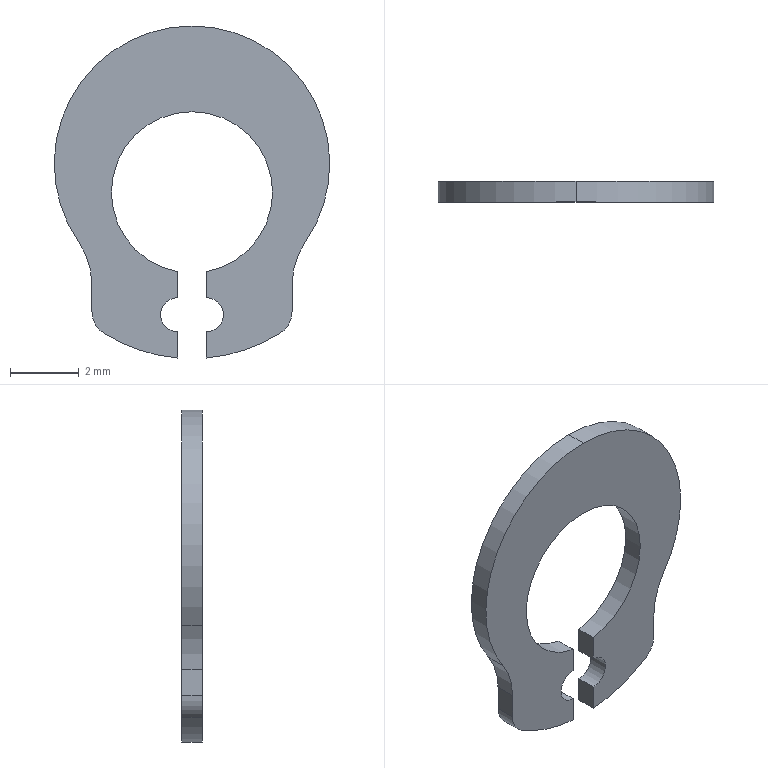Part | SolidWorks | features BaseBody 1 | 1 solid | 20 faces | box 8.033 x 0.6 x 9.682 mm | volume 24.423 mm3 | cylinder 12 | plane 8 | commonest cylinder face diameters 1 x2 1.5 x2 4.5 x2 4.7 x2 8.033 x2 9.7 x2
STEP:
#1=CARTESIAN_POINT('',(0.4167,-0.6,-2.313));
#2=VERTEX_POINT('',#1);
#3=CARTESIAN_POINT('',(0.,-0.6,2.35));
#4=VERTEX_POINT('',#3);
#5=CARTESIAN_POINT('',(0.,-0.6,0.));
#6=DIRECTION('',(0.,-1.,0.));
#7=DIRECTION('',(0.,0.,-1.));
#8=AXIS2_PLACEMENT_3D('',#5,#6,#7);
#9=CIRCLE('',#8,2.35);
#10=EDGE_CURVE('',#2,#4,#9,.T.);
#11=ORIENTED_EDGE('',*,*,#10,.T.);
#12=CARTESIAN_POINT('',(0.,0.,2.35));
#13=VERTEX_POINT('',#12);
#14=CARTESIAN_POINT('',(0.,-0.6,2.35));
#15=DIRECTION('',(0.,1.,0.));
#16=VECTOR('',#15,1000.);
#17=LINE('',#14,#16);
#18=EDGE_CURVE('',#4,#13,#17,.T.);
#19=ORIENTED_EDGE('',*,*,#18,.T.);
#20=CARTESIAN_POINT('',(0.4167,0.,-2.313));
#21=VERTEX_POINT('',#20);
#22=CARTESIAN_POINT('',(0.,0.,0.));
#23=DIRECTION('',(0.,-1.,0.));
#24=DIRECTION('',(0.,0.,-1.));
#25=AXIS2_PLACEMENT_3D('',#22,#23,#24);
#26=CIRCLE('',#25,2.35);
#27=EDGE_CURVE('',#21,#13,#26,.T.);
#28=ORIENTED_EDGE('',*,*,#27,.F.);
#29=CARTESIAN_POINT('',(0.4167,-0.6,-2.313));
#30=DIRECTION('',(0.,1.,0.));
#31=VECTOR('',#30,1000.);
#32=LINE('',#29,#31);
#33=EDGE_CURVE('',#2,#21,#32,.T.);
#34=ORIENTED_EDGE('',*,*,#33,.F.);
#35=EDGE_LOOP('',(#11,#19,#28,#34));
#36=FACE_OUTER_BOUND('',#35,.T.);
#37=CARTESIAN_POINT('',(0.,-0.6,0.));
#38=DIRECTION('',(0.,1.,0.));
#39=DIRECTION('',(0.,0.,1.));
#40=AXIS2_PLACEMENT_3D('',#37,#38,#39);
#41=CYLINDRICAL_SURFACE('',#40,2.35);
#42=ADVANCED_FACE('',(#36),#41,.F.);
#43=CARTESIAN_POINT('',(-3.312,-0.6,-1.44));
#44=VERTEX_POINT('',#43);
#45=CARTESIAN_POINT('',(0.,-0.6,4.85));
#46=VERTEX_POINT('',#45);
#47=CARTESIAN_POINT('',(0.,-0.6,0.8333));
#48=DIRECTION('',(0.,1.,0.));
#49=DIRECTION('',(0.,0.,-1.));
#50=AXIS2_PLACEMENT_3D('',#47,#48,#49);
#51=CIRCLE('',#50,4.017);
#52=EDGE_CURVE('',#44,#46,#51,.T.);
#53=ORIENTED_EDGE('',*,*,#52,.T.);
#54=CARTESIAN_POINT('',(0.,0.,4.85));
#55=VERTEX_POINT('',#54);
#56=CARTESIAN_POINT('',(0.,-0.6,4.85));
#57=DIRECTION('',(0.,1.,0.));
#58=VECTOR('',#57,1000.);
#59=LINE('',#56,#58);
#60=EDGE_CURVE('',#46,#55,#59,.T.);
#61=ORIENTED_EDGE('',*,*,#60,.T.);
#62=CARTESIAN_POINT('',(-3.312,0.,-1.44));
#63=VERTEX_POINT('',#62);
#64=CARTESIAN_POINT('',(0.,0.,0.8333));
#65=DIRECTION('',(0.,1.,0.));
#66=DIRECTION('',(0.,0.,-1.));
#67=AXIS2_PLACEMENT_3D('',#64,#65,#66);
#68=CIRCLE('',#67,4.017);
#69=EDGE_CURVE('',#63,#55,#68,.T.);
#70=ORIENTED_EDGE('',*,*,#69,.F.);
#71=CARTESIAN_POINT('',(-3.312,-0.6,-1.44));
#72=DIRECTION('',(0.,-1.,0.));
#73=VECTOR('',#72,1000.);
#74=LINE('',#71,#73);
#75=EDGE_CURVE('',#63,#44,#74,.T.);
#76=ORIENTED_EDGE('',*,*,#75,.T.);
#77=EDGE_LOOP('',(#53,#61,#70,#76));
#78=FACE_OUTER_BOUND('',#77,.T.);
#79=CARTESIAN_POINT('',(0.,-0.6,0.8333));
#80=DIRECTION('',(0.,1.,0.));
#81=DIRECTION('',(0.,0.,1.));
#82=AXIS2_PLACEMENT_3D('',#79,#80,#81);
#83=CYLINDRICAL_SURFACE('',#82,4.017);
#84=ADVANCED_FACE('',(#78),#83,.T.);
#85=CARTESIAN_POINT('',(-2.917,-0.6,-3.481));
#86=VERTEX_POINT('',#85);
#87=CARTESIAN_POINT('',(-2.563,-0.6,-4.117));
#88=VERTEX_POINT('',#87);
#89=CARTESIAN_POINT('',(-2.167,-0.6,-3.481));
#90=DIRECTION('',(0.,-1.,0.));
#91=DIRECTION('',(0.,0.,-1.));
#92=AXIS2_PLACEMENT_3D('',#89,#90,#91);
#93=CIRCLE('',#92,0.75);
#94=EDGE_CURVE('',#86,#88,#93,.T.);
#95=ORIENTED_EDGE('',*,*,#94,.F.);
#96=CARTESIAN_POINT('',(-2.917,0.,-3.481));
#97=VERTEX_POINT('',#96);
#98=CARTESIAN_POINT('',(-2.917,-0.6,-3.481));
#99=DIRECTION('',(0.,-1.,0.));
#100=VECTOR('',#99,1000.);
#101=LINE('',#98,#100);
#102=EDGE_CURVE('',#97,#86,#101,.T.);
#103=ORIENTED_EDGE('',*,*,#102,.F.);
#104=CARTESIAN_POINT('',(-2.563,0.,-4.117));
#105=VERTEX_POINT('',#104);
#106=CARTESIAN_POINT('',(-2.167,0.,-3.481));
#107=DIRECTION('',(0.,1.,0.));
#108=DIRECTION('',(0.,0.,-1.));
#109=AXIS2_PLACEMENT_3D('',#106,#107,#108);
#110=CIRCLE('',#109,0.75);
#111=EDGE_CURVE('',#105,#97,#110,.T.);
#112=ORIENTED_EDGE('',*,*,#111,.F.);
#113=CARTESIAN_POINT('',(-2.563,-0.6,-4.117));
#114=DIRECTION('',(0.,1.,0.));
#115=VECTOR('',#114,1000.);
#116=LINE('',#113,#115);
#117=EDGE_CURVE('',#88,#105,#116,.T.);
#118=ORIENTED_EDGE('',*,*,#117,.F.);
#119=EDGE_LOOP('',(#95,#103,#112,#118));
#120=FACE_OUTER_BOUND('',#119,.T.);
#121=CARTESIAN_POINT('',(-2.167,-0.6,-3.481));
#122=DIRECTION('',(0.,1.,0.));
#123=DIRECTION('',(0.,0.,1.));
#124=AXIS2_PLACEMENT_3D('',#121,#122,#123);
#125=CYLINDRICAL_SURFACE('',#124,0.75);
#126=ADVANCED_FACE('',(#120),#125,.T.);
#127=CARTESIAN_POINT('',(2.563,-0.6,-4.117));
#128=VERTEX_POINT('',#127);
#129=CARTESIAN_POINT('',(2.917,-0.6,-3.481));
#130=VERTEX_POINT('',#129);
#131=CARTESIAN_POINT('',(2.167,-0.6,-3.481));
#132=DIRECTION('',(0.,-1.,0.));
#133=DIRECTION('',(0.,0.,-1.));
#134=AXIS2_PLACEMENT_3D('',#131,#132,#133);
#135=CIRCLE('',#134,0.75);
#136=EDGE_CURVE('',#128,#130,#135,.T.);
#137=ORIENTED_EDGE('',*,*,#136,.F.);
#138=CARTESIAN_POINT('',(2.563,0.,-4.117));
#139=VERTEX_POINT('',#138);
#140=CARTESIAN_POINT('',(2.563,-0.6,-4.117));
#141=DIRECTION('',(0.,-1.,0.));
#142=VECTOR('',#141,1000.);
#143=LINE('',#140,#142);
#144=EDGE_CURVE('',#139,#128,#143,.T.);
#145=ORIENTED_EDGE('',*,*,#144,.F.);
#146=CARTESIAN_POINT('',(2.917,0.,-3.481));
#147=VERTEX_POINT('',#146);
#148=CARTESIAN_POINT('',(2.167,0.,-3.481));
#149=DIRECTION('',(0.,1.,0.));
#150=DIRECTION('',(0.,0.,-1.));
#151=AXIS2_PLACEMENT_3D('',#148,#149,#150);
#152=CIRCLE('',#151,0.75);
#153=EDGE_CURVE('',#147,#139,#152,.T.);
#154=ORIENTED_EDGE('',*,*,#153,.F.);
#155=CARTESIAN_POINT('',(2.917,-0.6,-3.481));
#156=DIRECTION('',(0.,1.,0.));
#157=VECTOR('',#156,1000.);
#158=LINE('',#155,#157);
#159=EDGE_CURVE('',#130,#147,#158,.T.);
#160=ORIENTED_EDGE('',*,*,#159,.F.);
#161=EDGE_LOOP('',(#137,#145,#154,#160));
#162=FACE_OUTER_BOUND('',#161,.T.);
#163=CARTESIAN_POINT('',(2.167,-0.6,-3.481));
#164=DIRECTION('',(0.,1.,0.));
#165=DIRECTION('',(0.,0.,1.));
#166=AXIS2_PLACEMENT_3D('',#163,#164,#165);
#167=CYLINDRICAL_SURFACE('',#166,0.75);
#168=ADVANCED_FACE('',(#162),#167,.T.);
#169=CARTESIAN_POINT('',(-2.917,-0.6,-2.713));
#170=VERTEX_POINT('',#169);
#171=CARTESIAN_POINT('',(-5.167,-0.6,-2.713));
#172=DIRECTION('',(0.,1.,0.));
#173=DIRECTION('',(0.,0.,-1.));
#174=AXIS2_PLACEMENT_3D('',#171,#172,#173);
#175=CIRCLE('',#174,2.25);
#176=EDGE_CURVE('',#44,#170,#175,.T.);
#177=ORIENTED_EDGE('',*,*,#176,.F.);
#178=ORIENTED_EDGE('',*,*,#75,.F.);
#179=CARTESIAN_POINT('',(-2.917,0.,-2.713));
#180=VERTEX_POINT('',#179);
#181=CARTESIAN_POINT('',(-5.167,0.,-2.713));
#182=DIRECTION('',(0.,-1.,0.));
#183=DIRECTION('',(0.,0.,-1.));
#184=AXIS2_PLACEMENT_3D('',#181,#182,#183);
#185=CIRCLE('',#184,2.25);
#186=EDGE_CURVE('',#180,#63,#185,.T.);
#187=ORIENTED_EDGE('',*,*,#186,.F.);
#188=CARTESIAN_POINT('',(-2.917,0.,-2.713));
#189=DIRECTION('',(0.,1.,0.));
#190=VECTOR('',#189,1000.);
#191=LINE('',#188,#190);
#192=EDGE_CURVE('',#170,#180,#191,.T.);
#193=ORIENTED_EDGE('',*,*,#192,.F.);
#194=EDGE_LOOP('',(#177,#178,#187,#193));
#195=FACE_OUTER_BOUND('',#194,.T.);
#196=CARTESIAN_POINT('',(-5.167,-0.6,-2.713));
#197=DIRECTION('',(0.,1.,0.));
#198=DIRECTION('',(0.,0.,1.));
#199=AXIS2_PLACEMENT_3D('',#196,#197,#198);
#200=CYLINDRICAL_SURFACE('',#199,2.25);
#201=ADVANCED_FACE('',(#195),#200,.F.);
#202=CARTESIAN_POINT('',(2.917,-0.6,-2.713));
#203=VERTEX_POINT('',#202);
#204=CARTESIAN_POINT('',(3.312,-0.6,-1.44));
#205=VERTEX_POINT('',#204);
#206=CARTESIAN_POINT('',(5.167,-0.6,-2.713));
#207=DIRECTION('',(0.,1.,0.));
#208=DIRECTION('',(0.,0.,-1.));
#209=AXIS2_PLACEMENT_3D('',#206,#207,#208);
#210=CIRCLE('',#209,2.25);
#211=EDGE_CURVE('',#203,#205,#210,.T.);
#212=ORIENTED_EDGE('',*,*,#211,.F.);
#213=CARTESIAN_POINT('',(2.917,0.,-2.713));
#214=VERTEX_POINT('',#213);
#215=CARTESIAN_POINT('',(2.917,-0.6,-2.713));
#216=DIRECTION('',(0.,-1.,0.));
#217=VECTOR('',#216,1000.);
#218=LINE('',#215,#217);
#219=EDGE_CURVE('',#214,#203,#218,.T.);
#220=ORIENTED_EDGE('',*,*,#219,.F.);
#221=CARTESIAN_POINT('',(3.312,0.,-1.44));
#222=VERTEX_POINT('',#221);
#223=CARTESIAN_POINT('',(5.167,0.,-2.713));
#224=DIRECTION('',(0.,-1.,0.));
#225=DIRECTION('',(0.,0.,-1.));
#226=AXIS2_PLACEMENT_3D('',#223,#224,#225);
#227=CIRCLE('',#226,2.25);
#228=EDGE_CURVE('',#222,#214,#227,.T.);
#229=ORIENTED_EDGE('',*,*,#228,.F.);
#230=CARTESIAN_POINT('',(3.312,-0.6,-1.44));
#231=DIRECTION('',(0.,1.,0.));
#232=VECTOR('',#231,1000.);
#233=LINE('',#230,#232);
#234=EDGE_CURVE('',#205,#222,#233,.T.);
#235=ORIENTED_EDGE('',*,*,#234,.F.);
#236=EDGE_LOOP('',(#212,#220,#229,#235));
#237=FACE_OUTER_BOUND('',#236,.T.);
#238=CARTESIAN_POINT('',(5.167,-0.6,-2.713));
#239=DIRECTION('',(0.,1.,0.));
#240=DIRECTION('',(0.,0.,1.));
#241=AXIS2_PLACEMENT_3D('',#238,#239,#240);
#242=CYLINDRICAL_SURFACE('',#241,2.25);
#243=ADVANCED_FACE('',(#237),#242,.F.);
#244=CARTESIAN_POINT('',(-0.4167,-0.6,-4.072));
#245=VERTEX_POINT('',#244);
#246=CARTESIAN_POINT('',(-0.4167,-0.6,-3.072));
#247=VERTEX_POINT('',#246);
#248=CARTESIAN_POINT('',(-0.4167,-0.6,-3.572));
#249=DIRECTION('',(0.,1.,0.));
#250=DIRECTION('',(0.,0.,-1.));
#251=AXIS2_PLACEMENT_3D('',#248,#249,#250);
#252=CIRCLE('',#251,0.5);
#253=EDGE_CURVE('',#245,#247,#252,.T.);
#254=ORIENTED_EDGE('',*,*,#253,.F.);
#255=CARTESIAN_POINT('',(-0.4167,0.,-4.072));
#256=VERTEX_POINT('',#255);
#257=CARTESIAN_POINT('',(-0.4167,11.995,-4.072));
#258=DIRECTION('',(0.,-1.,0.));
#259=VECTOR('',#258,1000.);
#260=LINE('',#257,#259);
#261=EDGE_CURVE('',#256,#245,#260,.T.);
#262=ORIENTED_EDGE('',*,*,#261,.F.);
#263=CARTESIAN_POINT('',(-0.4167,0.,-3.072));
#264=VERTEX_POINT('',#263);
#265=CARTESIAN_POINT('',(-0.4167,0.,-3.572));
#266=DIRECTION('',(0.,1.,0.));
#267=DIRECTION('',(0.,0.,-1.));
#268=AXIS2_PLACEMENT_3D('',#265,#266,#267);
#269=CIRCLE('',#268,0.5);
#270=EDGE_CURVE('',#256,#264,#269,.T.);
#271=ORIENTED_EDGE('',*,*,#270,.T.);
#272=CARTESIAN_POINT('',(-0.4167,11.995,-3.072));
#273=DIRECTION('',(0.,1.,0.));
#274=VECTOR('',#273,1000.);
#275=LINE('',#272,#274);
#276=EDGE_CURVE('',#247,#264,#275,.T.);
#277=ORIENTED_EDGE('',*,*,#276,.F.);
#278=EDGE_LOOP('',(#254,#262,#271,#277));
#279=FACE_OUTER_BOUND('',#278,.T.);
#280=CARTESIAN_POINT('',(-0.4167,11.995,-3.572));
#281=DIRECTION('',(0.,-1.,0.));
#282=DIRECTION('',(0.,0.,-1.));
#283=AXIS2_PLACEMENT_3D('',#280,#281,#282);
#284=CYLINDRICAL_SURFACE('',#283,0.5);
#285=ADVANCED_FACE('',(#279),#284,.F.);
#286=CARTESIAN_POINT('',(0.4167,-0.6,-3.072));
#287=VERTEX_POINT('',#286);
#288=CARTESIAN_POINT('',(0.4167,-0.6,-4.072));
#289=VERTEX_POINT('',#288);
#290=CARTESIAN_POINT('',(0.4167,-0.6,-3.572));
#291=DIRECTION('',(0.,1.,0.));
#292=DIRECTION('',(0.,0.,-1.));
#293=AXIS2_PLACEMENT_3D('',#290,#291,#292);
#294=CIRCLE('',#293,0.5);
#295=EDGE_CURVE('',#287,#289,#294,.T.);
#296=ORIENTED_EDGE('',*,*,#295,.F.);
#297=CARTESIAN_POINT('',(0.4167,0.,-3.072));
#298=VERTEX_POINT('',#297);
#299=CARTESIAN_POINT('',(0.4167,11.995,-3.072));
#300=DIRECTION('',(0.,-1.,0.));
#301=VECTOR('',#300,1000.);
#302=LINE('',#299,#301);
#303=EDGE_CURVE('',#298,#287,#302,.T.);
#304=ORIENTED_EDGE('',*,*,#303,.F.);
#305=CARTESIAN_POINT('',(0.4167,0.,-4.072));
#306=VERTEX_POINT('',#305);
#307=CARTESIAN_POINT('',(0.4167,0.,-3.572));
#308=DIRECTION('',(0.,1.,0.));
#309=DIRECTION('',(0.,0.,-1.));
#310=AXIS2_PLACEMENT_3D('',#307,#308,#309);
#311=CIRCLE('',#310,0.5);
#312=EDGE_CURVE('',#298,#306,#311,.T.);
#313=ORIENTED_EDGE('',*,*,#312,.T.);
#314=CARTESIAN_POINT('',(0.4167,11.995,-4.072));
#315=DIRECTION('',(0.,1.,0.));
#316=VECTOR('',#315,1000.);
#317=LINE('',#314,#316);
#318=EDGE_CURVE('',#289,#306,#317,.T.);
#319=ORIENTED_EDGE('',*,*,#318,.F.);
#320=EDGE_LOOP('',(#296,#304,#313,#319));
#321=FACE_OUTER_BOUND('',#320,.T.);
#322=CARTESIAN_POINT('',(0.4167,11.995,-3.572));
#323=DIRECTION('',(0.,-1.,0.));
#324=DIRECTION('',(0.,0.,-1.));
#325=AXIS2_PLACEMENT_3D('',#322,#323,#324);
#326=CYLINDRICAL_SURFACE('',#325,0.5);
#327=ADVANCED_FACE('',(#321),#326,.F.);
#328=CARTESIAN_POINT('',(-0.4167,0.,-4.832));
#329=VERTEX_POINT('',#328);
#330=CARTESIAN_POINT('',(0.,0.,0.));
#331=DIRECTION('',(0.,1.,0.));
#332=DIRECTION('',(1.,0.,0.));
#333=AXIS2_PLACEMENT_3D('',#330,#331,#332);
#334=CIRCLE('',#333,4.85);
#335=EDGE_CURVE('',#329,#105,#334,.T.);
#336=ORIENTED_EDGE('',*,*,#335,.T.);
#337=ORIENTED_EDGE('',*,*,#111,.T.);
#338=CARTESIAN_POINT('',(-2.917,0.,-1.928));
#339=DIRECTION('',(0.,0.,1.));
#340=VECTOR('',#339,1000.);
#341=LINE('',#338,#340);
#342=EDGE_CURVE('',#97,#180,#341,.T.);
#343=ORIENTED_EDGE('',*,*,#342,.T.);
#344=ORIENTED_EDGE('',*,*,#186,.T.);
#345=ORIENTED_EDGE('',*,*,#69,.T.);
#346=CARTESIAN_POINT('',(0.,0.,0.8333));
#347=DIRECTION('',(0.,1.,0.));
#348=DIRECTION('',(0.,0.,-1.));
#349=AXIS2_PLACEMENT_3D('',#346,#347,#348);
#350=CIRCLE('',#349,4.017);
#351=EDGE_CURVE('',#55,#222,#350,.T.);
#352=ORIENTED_EDGE('',*,*,#351,.T.);
#353=ORIENTED_EDGE('',*,*,#228,.T.);
#354=CARTESIAN_POINT('',(2.917,0.,-1.928));
#355=DIRECTION('',(0.,0.,-1.));
#356=VECTOR('',#355,1000.);
#357=LINE('',#354,#356);
#358=EDGE_CURVE('',#214,#147,#357,.T.);
#359=ORIENTED_EDGE('',*,*,#358,.T.);
#360=ORIENTED_EDGE('',*,*,#153,.T.);
#361=CARTESIAN_POINT('',(0.4167,0.,-4.832));
#362=VERTEX_POINT('',#361);
#363=CARTESIAN_POINT('',(0.,0.,0.));
#364=DIRECTION('',(0.,1.,0.));
#365=DIRECTION('',(1.,0.,0.));
#366=AXIS2_PLACEMENT_3D('',#363,#364,#365);
#367=CIRCLE('',#366,4.85);
#368=EDGE_CURVE('',#139,#362,#367,.T.);
#369=ORIENTED_EDGE('',*,*,#368,.T.);
#370=CARTESIAN_POINT('',(0.4167,0.,-2.313));
#371=DIRECTION('',(0.,0.,1.));
#372=VECTOR('',#371,1000.);
#373=LINE('',#370,#372);
#374=EDGE_CURVE('',#362,#306,#373,.T.);
#375=ORIENTED_EDGE('',*,*,#374,.T.);
#376=ORIENTED_EDGE('',*,*,#312,.F.);
#377=CARTESIAN_POINT('',(0.4167,0.,-2.313));
#378=DIRECTION('',(0.,0.,1.));
#379=VECTOR('',#378,1000.);
#380=LINE('',#377,#379);
#381=EDGE_CURVE('',#298,#21,#380,.T.);
#382=ORIENTED_EDGE('',*,*,#381,.T.);
#383=ORIENTED_EDGE('',*,*,#27,.T.);
#384=CARTESIAN_POINT('',(-0.4167,0.,-2.313));
#385=VERTEX_POINT('',#384);
#386=CARTESIAN_POINT('',(0.,0.,0.));
#387=DIRECTION('',(0.,-1.,0.));
#388=DIRECTION('',(0.,0.,-1.));
#389=AXIS2_PLACEMENT_3D('',#386,#387,#388);
#390=CIRCLE('',#389,2.35);
#391=EDGE_CURVE('',#13,#385,#390,.T.);
#392=ORIENTED_EDGE('',*,*,#391,.T.);
#393=CARTESIAN_POINT('',(-0.4167,0.,-2.313));
#394=DIRECTION('',(0.,0.,-1.));
#395=VECTOR('',#394,1000.);
#396=LINE('',#393,#395);
#397=EDGE_CURVE('',#385,#264,#396,.T.);
#398=ORIENTED_EDGE('',*,*,#397,.T.);
#399=ORIENTED_EDGE('',*,*,#270,.F.);
#400=CARTESIAN_POINT('',(-0.4167,0.,-2.313));
#401=DIRECTION('',(0.,0.,-1.));
#402=VECTOR('',#401,1000.);
#403=LINE('',#400,#402);
#404=EDGE_CURVE('',#256,#329,#403,.T.);
#405=ORIENTED_EDGE('',*,*,#404,.T.);
#406=EDGE_LOOP('',(#336,#337,#343,#344,#345,#352,#353,#359,#360,#369,#375,#376,#382,#383,#392,#398,#399,#405));
#407=FACE_OUTER_BOUND('',#406,.T.);
#408=CARTESIAN_POINT('',(0.,0.,0.));
#409=DIRECTION('',(0.,-1.,0.));
#410=DIRECTION('',(0.,0.,-1.));
#411=AXIS2_PLACEMENT_3D('',#408,#409,#410);
#412=PLANE('',#411);
#413=ADVANCED_FACE('',(#407),#412,.F.);
#414=CARTESIAN_POINT('',(-2.917,-0.6,-1.928));
#415=DIRECTION('',(0.,0.,1.));
#416=VECTOR('',#415,1000.);
#417=LINE('',#414,#416);
#418=EDGE_CURVE('',#86,#170,#417,.T.);
#419=ORIENTED_EDGE('',*,*,#418,.F.);
#420=ORIENTED_EDGE('',*,*,#94,.T.);
#421=CARTESIAN_POINT('',(-0.4167,-0.6,-4.832));
#422=VERTEX_POINT('',#421);
#423=CARTESIAN_POINT('',(0.,-0.6,0.));
#424=DIRECTION('',(0.,1.,0.));
#425=DIRECTION('',(1.,0.,0.));
#426=AXIS2_PLACEMENT_3D('',#423,#424,#425);
#427=CIRCLE('',#426,4.85);
#428=EDGE_CURVE('',#422,#88,#427,.T.);
#429=ORIENTED_EDGE('',*,*,#428,.F.);
#430=CARTESIAN_POINT('',(-0.4167,-0.6,-2.313));
#431=DIRECTION('',(0.,0.,-1.));
#432=VECTOR('',#431,1000.);
#433=LINE('',#430,#432);
#434=EDGE_CURVE('',#245,#422,#433,.T.);
#435=ORIENTED_EDGE('',*,*,#434,.F.);
#436=ORIENTED_EDGE('',*,*,#253,.T.);
#437=CARTESIAN_POINT('',(-0.4167,-0.6,-2.313));
#438=VERTEX_POINT('',#437);
#439=CARTESIAN_POINT('',(-0.4167,-0.6,-2.313));
#440=DIRECTION('',(0.,0.,-1.));
#441=VECTOR('',#440,1000.);
#442=LINE('',#439,#441);
#443=EDGE_CURVE('',#438,#247,#442,.T.);
#444=ORIENTED_EDGE('',*,*,#443,.F.);
#445=CARTESIAN_POINT('',(0.,-0.6,0.));
#446=DIRECTION('',(0.,-1.,0.));
#447=DIRECTION('',(0.,0.,-1.));
#448=AXIS2_PLACEMENT_3D('',#445,#446,#447);
#449=CIRCLE('',#448,2.35);
#450=EDGE_CURVE('',#4,#438,#449,.T.);
#451=ORIENTED_EDGE('',*,*,#450,.F.);
#452=ORIENTED_EDGE('',*,*,#10,.F.);
#453=CARTESIAN_POINT('',(0.4167,-0.6,-2.313));
#454=DIRECTION('',(0.,0.,1.));
#455=VECTOR('',#454,1000.);
#456=LINE('',#453,#455);
#457=EDGE_CURVE('',#287,#2,#456,.T.);
#458=ORIENTED_EDGE('',*,*,#457,.F.);
#459=ORIENTED_EDGE('',*,*,#295,.T.);
#460=CARTESIAN_POINT('',(0.4167,-0.6,-4.832));
#461=VERTEX_POINT('',#460);
#462=CARTESIAN_POINT('',(0.4167,-0.6,-2.313));
#463=DIRECTION('',(0.,0.,1.));
#464=VECTOR('',#463,1000.);
#465=LINE('',#462,#464);
#466=EDGE_CURVE('',#461,#289,#465,.T.);
#467=ORIENTED_EDGE('',*,*,#466,.F.);
#468=CARTESIAN_POINT('',(0.,-0.6,0.));
#469=DIRECTION('',(0.,1.,0.));
#470=DIRECTION('',(1.,0.,0.));
#471=AXIS2_PLACEMENT_3D('',#468,#469,#470);
#472=CIRCLE('',#471,4.85);
#473=EDGE_CURVE('',#128,#461,#472,.T.);
#474=ORIENTED_EDGE('',*,*,#473,.F.);
#475=ORIENTED_EDGE('',*,*,#136,.T.);
#476=CARTESIAN_POINT('',(2.917,-0.6,-1.928));
#477=DIRECTION('',(0.,0.,-1.));
#478=VECTOR('',#477,1000.);
#479=LINE('',#476,#478);
#480=EDGE_CURVE('',#203,#130,#479,.T.);
#481=ORIENTED_EDGE('',*,*,#480,.F.);
#482=ORIENTED_EDGE('',*,*,#211,.T.);
#483=CARTESIAN_POINT('',(0.,-0.6,0.8333));
#484=DIRECTION('',(0.,1.,0.));
#485=DIRECTION('',(0.,0.,-1.));
#486=AXIS2_PLACEMENT_3D('',#483,#484,#485);
#487=CIRCLE('',#486,4.017);
#488=EDGE_CURVE('',#46,#205,#487,.T.);
#489=ORIENTED_EDGE('',*,*,#488,.F.);
#490=ORIENTED_EDGE('',*,*,#52,.F.);
#491=ORIENTED_EDGE('',*,*,#176,.T.);
#492=EDGE_LOOP('',(#419,#420,#429,#435,#436,#444,#451,#452,#458,#459,#467,#474,#475,#481,#482,#489,#490,#491));
#493=FACE_OUTER_BOUND('',#492,.T.);
#494=CARTESIAN_POINT('',(0.,-0.6,0.));
#495=DIRECTION('',(0.,-1.,0.));
#496=DIRECTION('',(0.,0.,-1.));
#497=AXIS2_PLACEMENT_3D('',#494,#495,#496);
#498=PLANE('',#497);
#499=ADVANCED_FACE('',(#493),#498,.T.);
#500=ORIENTED_EDGE('',*,*,#368,.F.);
#501=ORIENTED_EDGE('',*,*,#144,.T.);
#502=ORIENTED_EDGE('',*,*,#473,.T.);
#503=CARTESIAN_POINT('',(0.4167,-0.6,-4.832));
#504=DIRECTION('',(0.,1.,0.));
#505=VECTOR('',#504,1000.);
#506=LINE('',#503,#505);
#507=EDGE_CURVE('',#461,#362,#506,.T.);
#508=ORIENTED_EDGE('',*,*,#507,.T.);
#509=EDGE_LOOP('',(#500,#501,#502,#508));
#510=FACE_OUTER_BOUND('',#509,.T.);
#511=CARTESIAN_POINT('',(0.,-0.6,0.));
#512=DIRECTION('',(0.,1.,0.));
#513=DIRECTION('',(0.,0.,1.));
#514=AXIS2_PLACEMENT_3D('',#511,#512,#513);
#515=CYLINDRICAL_SURFACE('',#514,4.85);
#516=ADVANCED_FACE('',(#510),#515,.T.);
#517=ORIENTED_EDGE('',*,*,#480,.T.);
#518=ORIENTED_EDGE('',*,*,#159,.T.);
#519=ORIENTED_EDGE('',*,*,#358,.F.);
#520=ORIENTED_EDGE('',*,*,#219,.T.);
#521=EDGE_LOOP('',(#517,#518,#519,#520));
#522=FACE_OUTER_BOUND('',#521,.T.);
#523=CARTESIAN_POINT('',(2.917,-0.6,-1.928));
#524=DIRECTION('',(1.,0.,0.));
#525=DIRECTION('',(0.,0.,-1.));
#526=AXIS2_PLACEMENT_3D('',#523,#524,#525);
#527=PLANE('',#526);
#528=ADVANCED_FACE('',(#522),#527,.T.);
#529=ORIENTED_EDGE('',*,*,#60,.F.);
#530=ORIENTED_EDGE('',*,*,#488,.T.);
#531=ORIENTED_EDGE('',*,*,#234,.T.);
#532=ORIENTED_EDGE('',*,*,#351,.F.);
#533=EDGE_LOOP('',(#529,#530,#531,#532));
#534=FACE_OUTER_BOUND('',#533,.T.);
#535=CARTESIAN_POINT('',(0.,-0.6,0.8333));
#536=DIRECTION('',(0.,1.,0.));
#537=DIRECTION('',(0.,0.,1.));
#538=AXIS2_PLACEMENT_3D('',#535,#536,#537);
#539=CYLINDRICAL_SURFACE('',#538,4.017);
#540=ADVANCED_FACE('',(#534),#539,.T.);
#541=ORIENTED_EDGE('',*,*,#342,.F.);
#542=ORIENTED_EDGE('',*,*,#102,.T.);
#543=ORIENTED_EDGE('',*,*,#418,.T.);
#544=ORIENTED_EDGE('',*,*,#192,.T.);
#545=EDGE_LOOP('',(#541,#542,#543,#544));
#546=FACE_OUTER_BOUND('',#545,.T.);
#547=CARTESIAN_POINT('',(-2.917,-0.6,-1.928));
#548=DIRECTION('',(-1.,0.,0.));
#549=DIRECTION('',(0.,1.,0.));
#550=AXIS2_PLACEMENT_3D('',#547,#548,#549);
#551=PLANE('',#550);
#552=ADVANCED_FACE('',(#546),#551,.T.);
#553=ORIENTED_EDGE('',*,*,#428,.T.);
#554=ORIENTED_EDGE('',*,*,#117,.T.);
#555=ORIENTED_EDGE('',*,*,#335,.F.);
#556=CARTESIAN_POINT('',(-0.4167,-0.6,-4.832));
#557=DIRECTION('',(0.,1.,0.));
#558=VECTOR('',#557,1000.);
#559=LINE('',#556,#558);
#560=EDGE_CURVE('',#422,#329,#559,.T.);
#561=ORIENTED_EDGE('',*,*,#560,.F.);
#562=EDGE_LOOP('',(#553,#554,#555,#561));
#563=FACE_OUTER_BOUND('',#562,.T.);
#564=CARTESIAN_POINT('',(0.,-0.6,0.));
#565=DIRECTION('',(0.,1.,0.));
#566=DIRECTION('',(0.,0.,1.));
#567=AXIS2_PLACEMENT_3D('',#564,#565,#566);
#568=CYLINDRICAL_SURFACE('',#567,4.85);
#569=ADVANCED_FACE('',(#563),#568,.T.);
#570=ORIENTED_EDGE('',*,*,#18,.F.);
#571=ORIENTED_EDGE('',*,*,#450,.T.);
#572=CARTESIAN_POINT('',(-0.4167,-0.6,-2.313));
#573=DIRECTION('',(0.,1.,0.));
#574=VECTOR('',#573,1000.);
#575=LINE('',#572,#574);
#576=EDGE_CURVE('',#438,#385,#575,.T.);
#577=ORIENTED_EDGE('',*,*,#576,.T.);
#578=ORIENTED_EDGE('',*,*,#391,.F.);
#579=EDGE_LOOP('',(#570,#571,#577,#578));
#580=FACE_OUTER_BOUND('',#579,.T.);
#581=CARTESIAN_POINT('',(0.,-0.6,0.));
#582=DIRECTION('',(0.,1.,0.));
#583=DIRECTION('',(0.,0.,1.));
#584=AXIS2_PLACEMENT_3D('',#581,#582,#583);
#585=CYLINDRICAL_SURFACE('',#584,2.35);
#586=ADVANCED_FACE('',(#580),#585,.F.);
#587=ORIENTED_EDGE('',*,*,#381,.F.);
#588=ORIENTED_EDGE('',*,*,#303,.T.);
#589=ORIENTED_EDGE('',*,*,#457,.T.);
#590=ORIENTED_EDGE('',*,*,#33,.T.);
#591=EDGE_LOOP('',(#587,#588,#589,#590));
#592=FACE_OUTER_BOUND('',#591,.T.);
#593=CARTESIAN_POINT('',(0.4167,-0.6,-2.313));
#594=DIRECTION('',(-1.,0.,0.));
#595=DIRECTION('',(0.,0.,1.));
#596=AXIS2_PLACEMENT_3D('',#593,#594,#595);
#597=PLANE('',#596);
#598=ADVANCED_FACE('',(#592),#597,.T.);
#599=ORIENTED_EDGE('',*,*,#466,.T.);
#600=ORIENTED_EDGE('',*,*,#318,.T.);
#601=ORIENTED_EDGE('',*,*,#374,.F.);
#602=ORIENTED_EDGE('',*,*,#507,.F.);
#603=EDGE_LOOP('',(#599,#600,#601,#602));
#604=FACE_OUTER_BOUND('',#603,.T.);
#605=CARTESIAN_POINT('',(0.4167,-0.6,-2.313));
#606=DIRECTION('',(-1.,0.,0.));
#607=DIRECTION('',(0.,0.,1.));
#608=AXIS2_PLACEMENT_3D('',#605,#606,#607);
#609=PLANE('',#608);
#610=ADVANCED_FACE('',(#604),#609,.T.);
#611=ORIENTED_EDGE('',*,*,#404,.F.);
#612=ORIENTED_EDGE('',*,*,#261,.T.);
#613=ORIENTED_EDGE('',*,*,#434,.T.);
#614=ORIENTED_EDGE('',*,*,#560,.T.);
#615=EDGE_LOOP('',(#611,#612,#613,#614));
#616=FACE_OUTER_BOUND('',#615,.T.);
#617=CARTESIAN_POINT('',(-0.4167,-0.6,-2.313));
#618=DIRECTION('',(1.,0.,0.));
#619=DIRECTION('',(0.,1.,0.));
#620=AXIS2_PLACEMENT_3D('',#617,#618,#619);
#621=PLANE('',#620);
#622=ADVANCED_FACE('',(#616),#621,.T.);
#623=ORIENTED_EDGE('',*,*,#443,.T.);
#624=ORIENTED_EDGE('',*,*,#276,.T.);
#625=ORIENTED_EDGE('',*,*,#397,.F.);
#626=ORIENTED_EDGE('',*,*,#576,.F.);
#627=EDGE_LOOP('',(#623,#624,#625,#626));
#628=FACE_OUTER_BOUND('',#627,.T.);
#629=CARTESIAN_POINT('',(-0.4167,-0.6,-2.313));
#630=DIRECTION('',(1.,0.,0.));
#631=DIRECTION('',(0.,1.,0.));
#632=AXIS2_PLACEMENT_3D('',#629,#630,#631);
#633=PLANE('',#632);
#634=ADVANCED_FACE('',(#628),#633,.T.);
#635=CLOSED_SHELL('',(#42,#84,#126,#168,#201,#243,#285,#327,#413,#499,#516,#528,#540,#552,#569,#586,#598,#610,#622,#634));
#636=MANIFOLD_SOLID_BREP('',#635);
#637=CARTESIAN_POINT('',(0.,0.,0.));
#638=DIRECTION('',(0.,0.,1.));
#639=DIRECTION('',(1.,0.,0.));
#640=AXIS2_PLACEMENT_3D('',#637,#638,#639);
#641=(LENGTH_UNIT()NAMED_UNIT(*)SI_UNIT(.MILLI.,.METRE.));
#642=UNCERTAINTY_MEASURE_WITH_UNIT(LENGTH_MEASURE(0.00001),#641,'','');
#643=(NAMED_UNIT(*)PLANE_ANGLE_UNIT()SI_UNIT($,.RADIAN.));
#644=(NAMED_UNIT(*)SI_UNIT($,.STERADIAN.)SOLID_ANGLE_UNIT());
#645=(GEOMETRIC_REPRESENTATION_CONTEXT(3)GLOBAL_UNCERTAINTY_ASSIGNED_CONTEXT((#642))GLOBAL_UNIT_ASSIGNED_CONTEXT((#641,#643,#644))REPRESENTATION_CONTEXT('',''));
#646=ADVANCED_BREP_SHAPE_REPRESENTATION('',(#636,#640),#645);